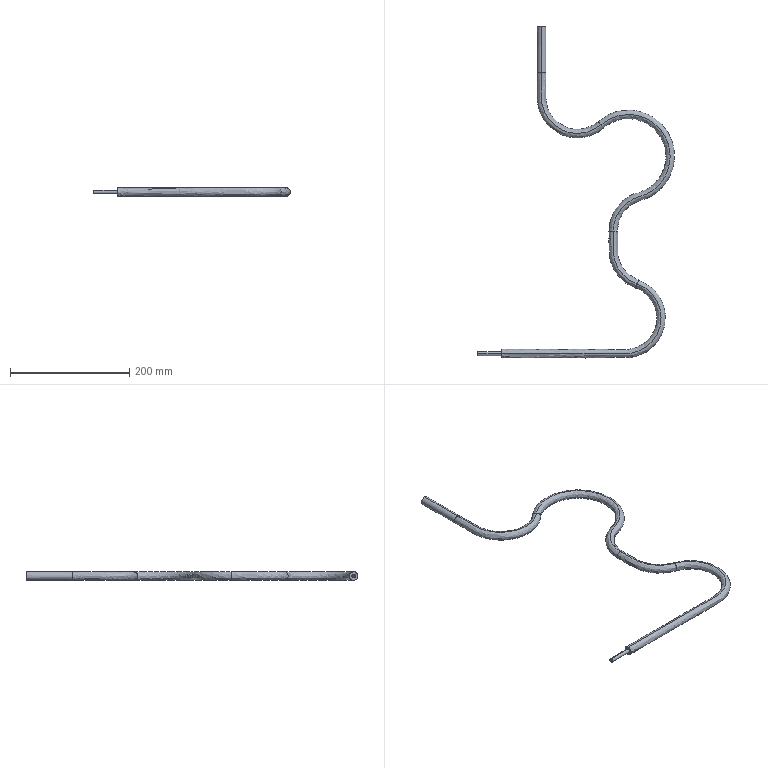Part | NX | features BREP 2 | 2 solids | 28 faces | box 329.489 x 555.807 x 14.509 mm | volume 142000 mm3 | spline 16 | cylinder 8 | plane 4 | commonest cylinder face diameters 6.35 x4 3.91 x2 14.5 x2